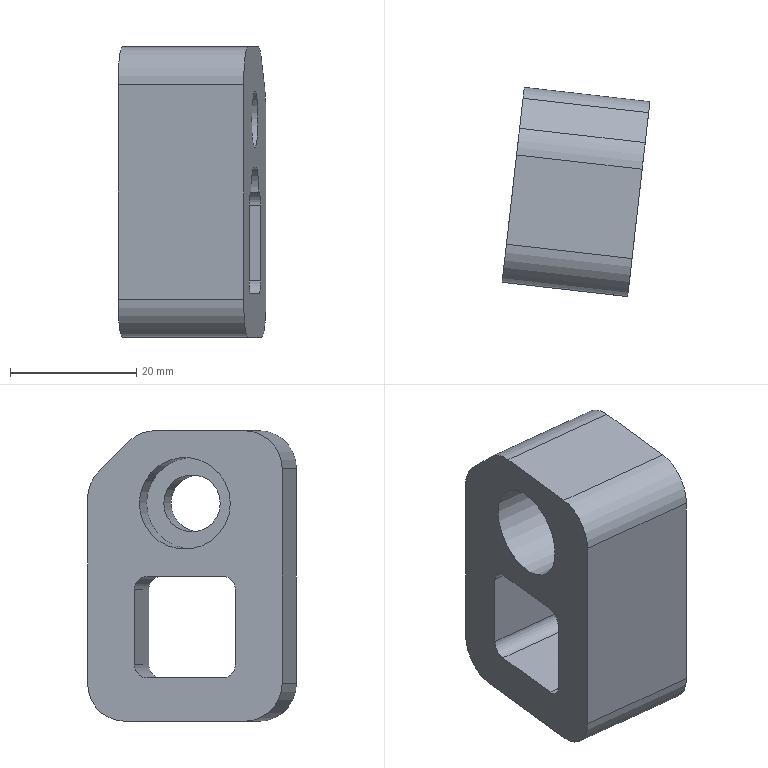Part | NX | features XQ 2 | 1 solid | 30 faces | box 23.381 x 33.065 x 46 mm | volume 19644 mm3 | plane 16 | cylinder 14 | commonest cylinder face diameters 12 x5 4.08 x4 8 x2 4 x1 9 x1 14.5 x1
STEP:
#1=CARTESIAN_POINT('',(3226.,-348.866,-101.287));
#2=VERTEX_POINT('',#1);
#3=CARTESIAN_POINT('',(3223.85,-367.744,-101.287));
#4=VERTEX_POINT('',#3);
#5=CARTESIAN_POINT('',(3230.269,-311.398,-101.287));
#6=DIRECTION('',(-0.1132,-0.9936,0.));
#7=VECTOR('',#6,1000.);
#8=LINE('',#5,#7);
#9=EDGE_CURVE('',#2,#4,#8,.T.);
#10=ORIENTED_EDGE('',*,*,#9,.T.);
#11=CARTESIAN_POINT('',(3223.17,-373.705,-95.287));
#12=VERTEX_POINT('',#11);
#13=CARTESIAN_POINT('',(3223.85,-367.744,-95.287));
#14=DIRECTION('',(-0.9936,0.1132,0.));
#15=DIRECTION('',(0.,0.,-1.));
#16=AXIS2_PLACEMENT_3D('',#13,#14,#15);
#17=CIRCLE('',#16,6.);
#18=EDGE_CURVE('',#4,#12,#17,.T.);
#19=ORIENTED_EDGE('',*,*,#18,.T.);
#20=CARTESIAN_POINT('',(3223.17,-373.705,-61.287));
#21=VERTEX_POINT('',#20);
#22=CARTESIAN_POINT('',(3223.17,-373.705,-144.775));
#23=DIRECTION('',(0.,0.,1.));
#24=VECTOR('',#23,1000.);
#25=LINE('',#22,#24);
#26=EDGE_CURVE('',#12,#21,#25,.T.);
#27=ORIENTED_EDGE('',*,*,#26,.T.);
#28=CARTESIAN_POINT('',(3223.85,-367.744,-55.287));
#29=VERTEX_POINT('',#28);
#30=CARTESIAN_POINT('',(3223.85,-367.744,-61.287));
#31=DIRECTION('',(-0.9936,0.1132,0.));
#32=DIRECTION('',(0.,0.,-1.));
#33=AXIS2_PLACEMENT_3D('',#30,#31,#32);
#34=CIRCLE('',#33,6.);
#35=EDGE_CURVE('',#21,#29,#34,.T.);
#36=ORIENTED_EDGE('',*,*,#35,.T.);
#37=CARTESIAN_POINT('',(3225.46,-353.614,-55.287));
#38=VERTEX_POINT('',#37);
#39=CARTESIAN_POINT('',(3230.269,-311.398,-55.287));
#40=DIRECTION('',(0.1132,0.9936,0.));
#41=VECTOR('',#40,1000.);
#42=LINE('',#39,#41);
#43=EDGE_CURVE('',#29,#38,#42,.T.);
#44=ORIENTED_EDGE('',*,*,#43,.T.);
#45=CARTESIAN_POINT('',(3225.94,-349.398,-57.044));
#46=VERTEX_POINT('',#45);
#47=CARTESIAN_POINT('',(3225.46,-353.614,-61.287));
#48=DIRECTION('',(-0.9936,0.1132,0.));
#49=DIRECTION('',(0.,0.,-1.));
#50=AXIS2_PLACEMENT_3D('',#47,#48,#49);
#51=CIRCLE('',#50,6.);
#52=EDGE_CURVE('',#38,#46,#51,.T.);
#53=ORIENTED_EDGE('',*,*,#52,.T.);
#54=CARTESIAN_POINT('',(3226.481,-344.651,-61.823));
#55=VERTEX_POINT('',#54);
#56=CARTESIAN_POINT('',(3233.07,-286.815,-120.033));
#57=DIRECTION('',(0.08005,0.7026,-0.7071));
#58=VECTOR('',#57,1000.);
#59=LINE('',#56,#58);
#60=EDGE_CURVE('',#46,#55,#59,.T.);
#61=ORIENTED_EDGE('',*,*,#60,.T.);
#62=CARTESIAN_POINT('',(3226.68,-342.905,-66.065));
#63=VERTEX_POINT('',#62);
#64=CARTESIAN_POINT('',(3226.,-348.866,-66.065));
#65=DIRECTION('',(-0.9936,0.1132,0.));
#66=DIRECTION('',(0.,0.,-1.));
#67=AXIS2_PLACEMENT_3D('',#64,#65,#66);
#68=CIRCLE('',#67,6.);
#69=EDGE_CURVE('',#55,#63,#68,.T.);
#70=ORIENTED_EDGE('',*,*,#69,.T.);
#71=CARTESIAN_POINT('',(3226.68,-342.905,-95.287));
#72=VERTEX_POINT('',#71);
#73=CARTESIAN_POINT('',(3226.68,-342.905,-144.775));
#74=DIRECTION('',(0.,0.,-1.));
#75=VECTOR('',#74,1000.);
#76=LINE('',#73,#75);
#77=EDGE_CURVE('',#63,#72,#76,.T.);
#78=ORIENTED_EDGE('',*,*,#77,.T.);
#79=CARTESIAN_POINT('',(3226.,-348.866,-95.287));
#80=DIRECTION('',(-0.9936,0.1132,0.));
#81=DIRECTION('',(0.,0.,-1.));
#82=AXIS2_PLACEMENT_3D('',#79,#80,#81);
#83=CIRCLE('',#82,6.);
#84=EDGE_CURVE('',#72,#2,#83,.T.);
#85=ORIENTED_EDGE('',*,*,#84,.T.);
#86=EDGE_LOOP('',(#10,#19,#27,#36,#44,#53,#61,#70,#78,#85));
#87=FACE_BOUND('',#86,.T.);
#88=CARTESIAN_POINT('',(3225.746,-351.102,-66.787));
#89=VERTEX_POINT('',#88);
#90=CARTESIAN_POINT('',(3224.925,-358.305,-66.787));
#91=DIRECTION('',(0.9936,-0.1132,0.));
#92=DIRECTION('',(0.1132,0.9936,0.));
#93=AXIS2_PLACEMENT_3D('',#90,#91,#92);
#94=CIRCLE('',#93,7.25);
#95=EDGE_CURVE('',#89,#89,#94,.T.);
#96=ORIENTED_EDGE('',*,*,#95,.T.);
#97=EDGE_LOOP('',(#96));
#98=FACE_BOUND('',#97,.T.);
#99=CARTESIAN_POINT('',(3225.604,-352.344,-78.322));
#100=VERTEX_POINT('',#99);
#101=CARTESIAN_POINT('',(3225.835,-350.317,-80.362));
#102=VERTEX_POINT('',#101);
#103=CARTESIAN_POINT('',(3225.604,-352.344,-80.362));
#104=DIRECTION('',(-0.9936,0.1132,0.));
#105=DIRECTION('',(0.,0.,-1.));
#106=AXIS2_PLACEMENT_3D('',#103,#104,#105);
#107=CIRCLE('',#106,2.04);
#108=EDGE_CURVE('',#100,#102,#107,.T.);
#109=ORIENTED_EDGE('',*,*,#108,.F.);
#110=CARTESIAN_POINT('',(3224.246,-364.266,-78.322));
#111=VERTEX_POINT('',#110);
#112=CARTESIAN_POINT('',(3230.269,-311.398,-78.322));
#113=DIRECTION('',(-0.1132,-0.9936,0.));
#114=VECTOR('',#113,1000.);
#115=LINE('',#112,#114);
#116=EDGE_CURVE('',#100,#111,#115,.T.);
#117=ORIENTED_EDGE('',*,*,#116,.T.);
#118=CARTESIAN_POINT('',(3224.015,-366.293,-80.362));
#119=VERTEX_POINT('',#118);
#120=CARTESIAN_POINT('',(3224.246,-364.266,-80.362));
#121=DIRECTION('',(-0.9936,0.1132,0.));
#122=DIRECTION('',(0.,0.,-1.));
#123=AXIS2_PLACEMENT_3D('',#120,#121,#122);
#124=CIRCLE('',#123,2.04);
#125=EDGE_CURVE('',#119,#111,#124,.T.);
#126=ORIENTED_EDGE('',*,*,#125,.F.);
#127=CARTESIAN_POINT('',(3224.015,-366.293,-92.362));
#128=VERTEX_POINT('',#127);
#129=CARTESIAN_POINT('',(3224.015,-366.293,-144.775));
#130=DIRECTION('',(0.,0.000000001,-1.));
#131=VECTOR('',#130,1000.);
#132=LINE('',#129,#131);
#133=EDGE_CURVE('',#119,#128,#132,.T.);
#134=ORIENTED_EDGE('',*,*,#133,.T.);
#135=CARTESIAN_POINT('',(3224.246,-364.266,-94.402));
#136=VERTEX_POINT('',#135);
#137=CARTESIAN_POINT('',(3224.246,-364.266,-92.362));
#138=DIRECTION('',(-0.9936,0.1132,0.));
#139=DIRECTION('',(0.,0.,-1.));
#140=AXIS2_PLACEMENT_3D('',#137,#138,#139);
#141=CIRCLE('',#140,2.04);
#142=EDGE_CURVE('',#136,#128,#141,.T.);
#143=ORIENTED_EDGE('',*,*,#142,.F.);
#144=CARTESIAN_POINT('',(3225.604,-352.344,-94.402));
#145=VERTEX_POINT('',#144);
#146=CARTESIAN_POINT('',(3230.269,-311.398,-94.402));
#147=DIRECTION('',(0.1132,0.9936,0.000000001));
#148=VECTOR('',#147,1000.);
#149=LINE('',#146,#148);
#150=EDGE_CURVE('',#136,#145,#149,.T.);
#151=ORIENTED_EDGE('',*,*,#150,.T.);
#152=CARTESIAN_POINT('',(3225.835,-350.317,-92.362));
#153=VERTEX_POINT('',#152);
#154=CARTESIAN_POINT('',(3225.604,-352.344,-92.362));
#155=DIRECTION('',(-0.9936,0.1132,0.));
#156=DIRECTION('',(0.,0.,-1.));
#157=AXIS2_PLACEMENT_3D('',#154,#155,#156);
#158=CIRCLE('',#157,2.04);
#159=EDGE_CURVE('',#153,#145,#158,.T.);
#160=ORIENTED_EDGE('',*,*,#159,.F.);
#161=CARTESIAN_POINT('',(3225.835,-350.317,-144.775));
#162=DIRECTION('',(0.,-0.000000001,1.));
#163=VECTOR('',#162,1000.);
#164=LINE('',#161,#163);
#165=EDGE_CURVE('',#153,#102,#164,.T.);
#166=ORIENTED_EDGE('',*,*,#165,.T.);
#167=EDGE_LOOP('',(#109,#117,#126,#134,#143,#151,#160,#166));
#168=FACE_BOUND('',#167,.T.);
#169=CARTESIAN_POINT('',(3230.269,-311.398,-144.775));
#170=DIRECTION('',(-0.9936,0.1132,0.));
#171=DIRECTION('',(-0.1132,-0.9936,0.));
#172=AXIS2_PLACEMENT_3D('',#169,#170,#171);
#173=PLANE('',#172);
#174=ADVANCED_FACE('',(#87,#98,#168),#173,.T.);
#175=CARTESIAN_POINT('',(3236.678,-361.154,-74.287));
#176=VERTEX_POINT('',#175);
#177=CARTESIAN_POINT('',(3236.225,-365.128,-78.322));
#178=VERTEX_POINT('',#177);
#179=CARTESIAN_POINT('',(3236.678,-361.154,-78.287));
#180=DIRECTION('',(0.9936,-0.1132,0.));
#181=DIRECTION('',(0.,0.,1.));
#182=AXIS2_PLACEMENT_3D('',#179,#180,#181);
#183=CIRCLE('',#182,4.);
#184=EDGE_CURVE('',#176,#178,#183,.T.);
#185=ORIENTED_EDGE('',*,*,#184,.T.);
#186=CARTESIAN_POINT('',(3236.452,-363.141,-78.322));
#187=VERTEX_POINT('',#186);
#188=CARTESIAN_POINT('',(3228.296,-434.719,-78.322));
#189=DIRECTION('',(0.1132,0.9936,0.));
#190=VECTOR('',#189,1000.);
#191=LINE('',#188,#190);
#192=EDGE_CURVE('',#178,#187,#191,.T.);
#193=ORIENTED_EDGE('',*,*,#192,.T.);
#194=CARTESIAN_POINT('',(3236.452,-363.141,-76.322));
#195=VERTEX_POINT('',#194);
#196=CARTESIAN_POINT('',(3236.452,-363.141,-68.563));
#197=DIRECTION('',(0.,0.,-1.));
#198=VECTOR('',#197,1000.);
#199=LINE('',#196,#198);
#200=EDGE_CURVE('',#195,#187,#199,.T.);
#201=ORIENTED_EDGE('',*,*,#200,.F.);
#202=CARTESIAN_POINT('',(3237.244,-356.186,-76.322));
#203=VERTEX_POINT('',#202);
#204=CARTESIAN_POINT('',(3237.471,-354.199,-76.322));
#205=DIRECTION('',(0.1132,0.9936,0.));
#206=VECTOR('',#205,1000.);
#207=LINE('',#204,#206);
#208=EDGE_CURVE('',#195,#203,#207,.T.);
#209=ORIENTED_EDGE('',*,*,#208,.T.);
#210=CARTESIAN_POINT('',(3237.244,-356.186,-78.322));
#211=VERTEX_POINT('',#210);
#212=CARTESIAN_POINT('',(3237.244,-356.186,-68.563));
#213=DIRECTION('',(0.,0.,-1.));
#214=VECTOR('',#213,1000.);
#215=LINE('',#212,#214);
#216=EDGE_CURVE('',#203,#211,#215,.T.);
#217=ORIENTED_EDGE('',*,*,#216,.T.);
#218=CARTESIAN_POINT('',(3237.47,-354.199,-78.322));
#219=VERTEX_POINT('',#218);
#220=CARTESIAN_POINT('',(3228.296,-434.719,-78.322));
#221=DIRECTION('',(0.1132,0.9936,0.));
#222=VECTOR('',#221,1000.);
#223=LINE('',#220,#222);
#224=EDGE_CURVE('',#211,#219,#223,.T.);
#225=ORIENTED_EDGE('',*,*,#224,.T.);
#226=CARTESIAN_POINT('',(3237.018,-358.173,-74.287));
#227=VERTEX_POINT('',#226);
#228=CARTESIAN_POINT('',(3237.018,-358.173,-78.287));
#229=DIRECTION('',(0.9936,-0.1132,0.));
#230=DIRECTION('',(0.,0.,1.));
#231=AXIS2_PLACEMENT_3D('',#228,#229,#230);
#232=CIRCLE('',#231,4.);
#233=EDGE_CURVE('',#219,#227,#232,.T.);
#234=ORIENTED_EDGE('',*,*,#233,.T.);
#235=CARTESIAN_POINT('',(3237.471,-354.199,-74.287));
#236=DIRECTION('',(-0.1132,-0.9936,0.));
#237=VECTOR('',#236,1000.);
#238=LINE('',#235,#237);
#239=EDGE_CURVE('',#227,#176,#238,.T.);
#240=ORIENTED_EDGE('',*,*,#239,.T.);
#241=EDGE_LOOP('',(#185,#193,#201,#209,#217,#225,#234,#240));
#242=FACE_BOUND('',#241,.T.);
#243=CARTESIAN_POINT('',(3228.296,-434.719,-68.563));
#244=DIRECTION('',(0.9936,-0.1132,0.));
#245=DIRECTION('',(0.1132,0.9936,0.));
#246=AXIS2_PLACEMENT_3D('',#243,#244,#245);
#247=PLANE('',#246);
#248=ADVANCED_FACE('',(#242),#247,.T.);
#249=CARTESIAN_POINT('',(3244.174,-366.034,-78.322));
#250=VERTEX_POINT('',#249);
#251=CARTESIAN_POINT('',(3283.917,-370.562,-78.322));
#252=DIRECTION('',(0.9936,-0.1132,0.));
#253=VECTOR('',#252,1000.);
#254=LINE('',#251,#253);
#255=EDGE_CURVE('',#178,#250,#254,.T.);
#256=ORIENTED_EDGE('',*,*,#255,.F.);
#257=ORIENTED_EDGE('',*,*,#184,.F.);
#258=CARTESIAN_POINT('',(3244.627,-362.059,-74.287));
#259=VERTEX_POINT('',#258);
#260=CARTESIAN_POINT('',(3284.37,-366.588,-74.287));
#261=DIRECTION('',(-0.9936,0.1132,0.));
#262=VECTOR('',#261,1000.);
#263=LINE('',#260,#262);
#264=EDGE_CURVE('',#259,#176,#263,.T.);
#265=ORIENTED_EDGE('',*,*,#264,.F.);
#266=CARTESIAN_POINT('',(3244.627,-362.059,-78.287));
#267=DIRECTION('',(-0.9936,0.1132,0.));
#268=DIRECTION('',(0.,0.,1.));
#269=AXIS2_PLACEMENT_3D('',#266,#267,#268);
#270=CIRCLE('',#269,4.);
#271=EDGE_CURVE('',#250,#259,#270,.T.);
#272=ORIENTED_EDGE('',*,*,#271,.F.);
#273=EDGE_LOOP('',(#256,#257,#265,#272));
#274=FACE_BOUND('',#273,.T.);
#275=CARTESIAN_POINT('',(3284.37,-366.588,-78.287));
#276=DIRECTION('',(0.9936,-0.1132,0.));
#277=DIRECTION('',(0.,0.,1.));
#278=AXIS2_PLACEMENT_3D('',#275,#276,#277);
#279=CYLINDRICAL_SURFACE('',#278,4.);
#280=ADVANCED_FACE('',(#274),#279,.F.);
#281=CARTESIAN_POINT('',(3245.419,-355.105,-78.322));
#282=VERTEX_POINT('',#281);
#283=CARTESIAN_POINT('',(3285.162,-359.633,-78.322));
#284=DIRECTION('',(-0.9936,0.1132,0.));
#285=VECTOR('',#284,1000.);
#286=LINE('',#283,#285);
#287=EDGE_CURVE('',#282,#219,#286,.T.);
#288=ORIENTED_EDGE('',*,*,#287,.F.);
#289=CARTESIAN_POINT('',(3244.966,-359.079,-74.287));
#290=VERTEX_POINT('',#289);
#291=CARTESIAN_POINT('',(3244.966,-359.079,-78.287));
#292=DIRECTION('',(-0.9936,0.1132,0.));
#293=DIRECTION('',(0.,0.,1.));
#294=AXIS2_PLACEMENT_3D('',#291,#292,#293);
#295=CIRCLE('',#294,4.);
#296=EDGE_CURVE('',#290,#282,#295,.T.);
#297=ORIENTED_EDGE('',*,*,#296,.F.);
#298=CARTESIAN_POINT('',(3284.709,-363.607,-74.287));
#299=DIRECTION('',(0.9936,-0.1132,0.));
#300=VECTOR('',#299,1000.);
#301=LINE('',#298,#300);
#302=EDGE_CURVE('',#227,#290,#301,.T.);
#303=ORIENTED_EDGE('',*,*,#302,.F.);
#304=ORIENTED_EDGE('',*,*,#233,.F.);
#305=EDGE_LOOP('',(#288,#297,#303,#304));
#306=FACE_BOUND('',#305,.T.);
#307=CARTESIAN_POINT('',(3284.709,-363.607,-78.287));
#308=DIRECTION('',(-0.9936,0.1132,0.));
#309=DIRECTION('',(0.,0.,-1.));
#310=AXIS2_PLACEMENT_3D('',#307,#308,#309);
#311=CYLINDRICAL_SURFACE('',#310,4.);
#312=ADVANCED_FACE('',(#306),#311,.F.);
#313=CARTESIAN_POINT('',(3245.476,-354.608,-78.322));
#314=VERTEX_POINT('',#313);
#315=CARTESIAN_POINT('',(3245.419,-355.104,-78.322));
#316=DIRECTION('',(-0.1132,-0.9936,0.));
#317=VECTOR('',#316,1000.);
#318=LINE('',#315,#317);
#319=EDGE_CURVE('',#314,#282,#318,.T.);
#320=ORIENTED_EDGE('',*,*,#319,.F.);
#321=CARTESIAN_POINT('',(3245.707,-352.581,-80.362));
#322=VERTEX_POINT('',#321);
#323=CARTESIAN_POINT('',(3245.476,-354.608,-80.362));
#324=DIRECTION('',(-0.9936,0.1132,0.));
#325=DIRECTION('',(0.,0.,1.));
#326=AXIS2_PLACEMENT_3D('',#323,#324,#325);
#327=CIRCLE('',#326,2.04);
#328=EDGE_CURVE('',#314,#322,#327,.T.);
#329=ORIENTED_EDGE('',*,*,#328,.T.);
#330=CARTESIAN_POINT('',(3245.707,-352.581,-92.362));
#331=VERTEX_POINT('',#330);
#332=CARTESIAN_POINT('',(3245.707,-352.581,-92.362));
#333=DIRECTION('',(0.,-0.000000001,1.));
#334=VECTOR('',#333,1000.);
#335=LINE('',#332,#334);
#336=EDGE_CURVE('',#331,#322,#335,.T.);
#337=ORIENTED_EDGE('',*,*,#336,.F.);
#338=CARTESIAN_POINT('',(3245.476,-354.608,-94.402));
#339=VERTEX_POINT('',#338);
#340=CARTESIAN_POINT('',(3245.476,-354.608,-92.362));
#341=DIRECTION('',(-0.9936,0.1132,0.));
#342=DIRECTION('',(0.,0.,1.));
#343=AXIS2_PLACEMENT_3D('',#340,#341,#342);
#344=CIRCLE('',#343,2.04);
#345=EDGE_CURVE('',#331,#339,#344,.T.);
#346=ORIENTED_EDGE('',*,*,#345,.T.);
#347=CARTESIAN_POINT('',(3244.117,-366.531,-94.402));
#348=VERTEX_POINT('',#347);
#349=CARTESIAN_POINT('',(3244.117,-366.531,-94.402));
#350=DIRECTION('',(0.1132,0.9936,0.000000001));
#351=VECTOR('',#350,1000.);
#352=LINE('',#349,#351);
#353=EDGE_CURVE('',#348,#339,#352,.T.);
#354=ORIENTED_EDGE('',*,*,#353,.F.);
#355=CARTESIAN_POINT('',(3243.886,-368.557,-92.362));
#356=VERTEX_POINT('',#355);
#357=CARTESIAN_POINT('',(3244.117,-366.531,-92.362));
#358=DIRECTION('',(-0.9936,0.1132,0.));
#359=DIRECTION('',(0.,0.,1.));
#360=AXIS2_PLACEMENT_3D('',#357,#358,#359);
#361=CIRCLE('',#360,2.04);
#362=EDGE_CURVE('',#348,#356,#361,.T.);
#363=ORIENTED_EDGE('',*,*,#362,.T.);
#364=CARTESIAN_POINT('',(3243.886,-368.557,-80.362));
#365=VERTEX_POINT('',#364);
#366=CARTESIAN_POINT('',(3243.886,-368.557,-80.362));
#367=DIRECTION('',(0.,0.000000001,-1.));
#368=VECTOR('',#367,1000.);
#369=LINE('',#366,#368);
#370=EDGE_CURVE('',#365,#356,#369,.T.);
#371=ORIENTED_EDGE('',*,*,#370,.F.);
#372=CARTESIAN_POINT('',(3244.117,-366.531,-78.322));
#373=VERTEX_POINT('',#372);
#374=CARTESIAN_POINT('',(3244.117,-366.531,-80.362));
#375=DIRECTION('',(-0.9936,0.1132,0.));
#376=DIRECTION('',(0.,0.,1.));
#377=AXIS2_PLACEMENT_3D('',#374,#375,#376);
#378=CIRCLE('',#377,2.04);
#379=EDGE_CURVE('',#365,#373,#378,.T.);
#380=ORIENTED_EDGE('',*,*,#379,.T.);
#381=CARTESIAN_POINT('',(3245.419,-355.104,-78.322));
#382=DIRECTION('',(-0.1132,-0.9936,0.));
#383=VECTOR('',#382,1000.);
#384=LINE('',#381,#383);
#385=EDGE_CURVE('',#250,#373,#384,.T.);
#386=ORIENTED_EDGE('',*,*,#385,.F.);
#387=ORIENTED_EDGE('',*,*,#271,.T.);
#388=CARTESIAN_POINT('',(3245.419,-355.104,-74.287));
#389=DIRECTION('',(-0.1132,-0.9936,0.));
#390=VECTOR('',#389,1000.);
#391=LINE('',#388,#390);
#392=EDGE_CURVE('',#290,#259,#391,.T.);
#393=ORIENTED_EDGE('',*,*,#392,.F.);
#394=ORIENTED_EDGE('',*,*,#296,.T.);
#395=EDGE_LOOP('',(#320,#329,#337,#346,#354,#363,#371,#380,#386,#387,#393,#394));
#396=FACE_BOUND('',#395,.T.);
#397=CARTESIAN_POINT('',(3243.042,-375.969,-61.287));
#398=VERTEX_POINT('',#397);
#399=CARTESIAN_POINT('',(3243.042,-375.969,-95.287));
#400=VERTEX_POINT('',#399);
#401=CARTESIAN_POINT('',(3243.042,-375.969,-68.563));
#402=DIRECTION('',(0.,0.,-1.));
#403=VECTOR('',#402,1000.);
#404=LINE('',#401,#403);
#405=EDGE_CURVE('',#398,#400,#404,.T.);
#406=ORIENTED_EDGE('',*,*,#405,.T.);
#407=CARTESIAN_POINT('',(3243.721,-370.008,-101.287));
#408=VERTEX_POINT('',#407);
#409=CARTESIAN_POINT('',(3243.721,-370.008,-95.287));
#410=DIRECTION('',(0.9936,-0.1132,0.));
#411=DIRECTION('',(0.,0.,1.));
#412=AXIS2_PLACEMENT_3D('',#409,#410,#411);
#413=CIRCLE('',#412,6.);
#414=EDGE_CURVE('',#400,#408,#413,.T.);
#415=ORIENTED_EDGE('',*,*,#414,.T.);
#416=CARTESIAN_POINT('',(3245.872,-351.13,-101.287));
#417=VERTEX_POINT('',#416);
#418=CARTESIAN_POINT('',(3236.245,-435.624,-101.287));
#419=DIRECTION('',(0.1132,0.9936,0.));
#420=VECTOR('',#419,1000.);
#421=LINE('',#418,#420);
#422=EDGE_CURVE('',#408,#417,#421,.T.);
#423=ORIENTED_EDGE('',*,*,#422,.T.);
#424=CARTESIAN_POINT('',(3246.551,-345.169,-95.287));
#425=VERTEX_POINT('',#424);
#426=CARTESIAN_POINT('',(3245.872,-351.13,-95.287));
#427=DIRECTION('',(0.9936,-0.1132,0.));
#428=DIRECTION('',(0.,0.,1.));
#429=AXIS2_PLACEMENT_3D('',#426,#427,#428);
#430=CIRCLE('',#429,6.);
#431=EDGE_CURVE('',#417,#425,#430,.T.);
#432=ORIENTED_EDGE('',*,*,#431,.T.);
#433=CARTESIAN_POINT('',(3246.551,-345.169,-66.065));
#434=VERTEX_POINT('',#433);
#435=CARTESIAN_POINT('',(3246.551,-345.169,-68.563));
#436=DIRECTION('',(0.,0.,1.));
#437=VECTOR('',#436,1000.);
#438=LINE('',#435,#437);
#439=EDGE_CURVE('',#425,#434,#438,.T.);
#440=ORIENTED_EDGE('',*,*,#439,.T.);
#441=CARTESIAN_POINT('',(3246.352,-346.915,-61.823));
#442=VERTEX_POINT('',#441);
#443=CARTESIAN_POINT('',(3245.872,-351.13,-66.065));
#444=DIRECTION('',(0.9936,-0.1132,0.));
#445=DIRECTION('',(0.,0.,1.));
#446=AXIS2_PLACEMENT_3D('',#443,#444,#445);
#447=CIRCLE('',#446,6.);
#448=EDGE_CURVE('',#434,#442,#447,.T.);
#449=ORIENTED_EDGE('',*,*,#448,.T.);
#450=CARTESIAN_POINT('',(3245.811,-351.662,-57.044));
#451=VERTEX_POINT('',#450);
#452=CARTESIAN_POINT('',(3241.68,-387.921,-20.551));
#453=DIRECTION('',(-0.08005,-0.7026,0.7071));
#454=VECTOR('',#453,1000.);
#455=LINE('',#452,#454);
#456=EDGE_CURVE('',#442,#451,#455,.T.);
#457=ORIENTED_EDGE('',*,*,#456,.T.);
#458=CARTESIAN_POINT('',(3245.331,-355.878,-55.287));
#459=VERTEX_POINT('',#458);
#460=CARTESIAN_POINT('',(3245.331,-355.878,-61.287));
#461=DIRECTION('',(0.9936,-0.1132,0.));
#462=DIRECTION('',(0.,0.,1.));
#463=AXIS2_PLACEMENT_3D('',#460,#461,#462);
#464=CIRCLE('',#463,6.);
#465=EDGE_CURVE('',#451,#459,#464,.T.);
#466=ORIENTED_EDGE('',*,*,#465,.T.);
#467=CARTESIAN_POINT('',(3243.721,-370.008,-55.287));
#468=VERTEX_POINT('',#467);
#469=CARTESIAN_POINT('',(3236.245,-435.624,-55.287));
#470=DIRECTION('',(-0.1132,-0.9936,0.));
#471=VECTOR('',#470,1000.);
#472=LINE('',#469,#471);
#473=EDGE_CURVE('',#459,#468,#472,.T.);
#474=ORIENTED_EDGE('',*,*,#473,.T.);
#475=CARTESIAN_POINT('',(3243.721,-370.008,-61.287));
#476=DIRECTION('',(0.9936,-0.1132,0.));
#477=DIRECTION('',(0.,0.,1.));
#478=AXIS2_PLACEMENT_3D('',#475,#476,#477);
#479=CIRCLE('',#478,6.);
#480=EDGE_CURVE('',#468,#398,#479,.T.);
#481=ORIENTED_EDGE('',*,*,#480,.T.);
#482=EDGE_LOOP('',(#406,#415,#423,#432,#440,#449,#457,#466,#474,#481));
#483=FACE_BOUND('',#482,.T.);
#484=CARTESIAN_POINT('',(3244.287,-365.04,-66.787));
#485=VERTEX_POINT('',#484);
#486=CARTESIAN_POINT('',(3244.796,-360.569,-66.787));
#487=DIRECTION('',(0.9936,-0.1132,0.));
#488=DIRECTION('',(-0.1132,-0.9936,0.));
#489=AXIS2_PLACEMENT_3D('',#486,#487,#488);
#490=CIRCLE('',#489,4.5);
#491=EDGE_CURVE('',#485,#485,#490,.T.);
#492=ORIENTED_EDGE('',*,*,#491,.F.);
#493=EDGE_LOOP('',(#492));
#494=FACE_BOUND('',#493,.T.);
#495=CARTESIAN_POINT('',(3236.245,-435.624,-68.563));
#496=DIRECTION('',(0.9936,-0.1132,0.));
#497=DIRECTION('',(0.1132,0.9936,0.));
#498=AXIS2_PLACEMENT_3D('',#495,#496,#497);
#499=PLANE('',#498);
#500=ADVANCED_FACE('',(#396,#483,#494),#499,.T.);
#501=ORIENTED_EDGE('',*,*,#422,.F.);
#502=CARTESIAN_POINT('',(3218.882,-367.178,-101.287));
#503=DIRECTION('',(-0.9936,0.1132,0.));
#504=VECTOR('',#503,1000.);
#505=LINE('',#502,#504);
#506=EDGE_CURVE('',#408,#4,#505,.T.);
#507=ORIENTED_EDGE('',*,*,#506,.T.);
#508=ORIENTED_EDGE('',*,*,#9,.F.);
#509=CARTESIAN_POINT('',(3221.033,-348.3,-101.287));
#510=DIRECTION('',(0.9936,-0.1132,0.));
#511=VECTOR('',#510,1000.);
#512=LINE('',#509,#511);
#513=EDGE_CURVE('',#2,#417,#512,.T.);
#514=ORIENTED_EDGE('',*,*,#513,.T.);
#515=EDGE_LOOP('',(#501,#507,#508,#514));
#516=FACE_BOUND('',#515,.T.);
#517=CARTESIAN_POINT('',(3219.957,-357.739,-101.287));
#518=DIRECTION('',(0.,0.,-1.));
#519=DIRECTION('',(-0.9588,0.284,0.));
#520=AXIS2_PLACEMENT_3D('',#517,#518,#519);
#521=PLANE('',#520);
#522=ADVANCED_FACE('',(#516),#521,.T.);
#523=ORIENTED_EDGE('',*,*,#26,.F.);
#524=CARTESIAN_POINT('',(3218.203,-373.139,-95.287));
#525=DIRECTION('',(0.9936,-0.1132,0.));
#526=VECTOR('',#525,1000.);
#527=LINE('',#524,#526);
#528=EDGE_CURVE('',#12,#400,#527,.T.);
#529=ORIENTED_EDGE('',*,*,#528,.T.);
#530=ORIENTED_EDGE('',*,*,#405,.F.);
#531=CARTESIAN_POINT('',(3218.203,-373.139,-61.287));
#532=DIRECTION('',(-0.9936,0.1132,0.));
#533=VECTOR('',#532,1000.);
#534=LINE('',#531,#533);
#535=EDGE_CURVE('',#398,#21,#534,.T.);
#536=ORIENTED_EDGE('',*,*,#535,.T.);
#537=EDGE_LOOP('',(#523,#529,#530,#536));
#538=FACE_BOUND('',#537,.T.);
#539=CARTESIAN_POINT('',(3218.203,-373.139,-86.362));
#540=DIRECTION('',(-0.1132,-0.9936,0.));
#541=DIRECTION('',(0.9936,-0.1132,0.));
#542=AXIS2_PLACEMENT_3D('',#539,#540,#541);
#543=PLANE('',#542);
#544=ADVANCED_FACE('',(#538),#543,.T.);
#545=ORIENTED_EDGE('',*,*,#439,.F.);
#546=CARTESIAN_POINT('',(3221.712,-342.339,-95.287));
#547=DIRECTION('',(-0.9936,0.1132,0.));
#548=VECTOR('',#547,1000.);
#549=LINE('',#546,#548);
#550=EDGE_CURVE('',#425,#72,#549,.T.);
#551=ORIENTED_EDGE('',*,*,#550,.T.);
#552=ORIENTED_EDGE('',*,*,#77,.F.);
#553=CARTESIAN_POINT('',(3221.712,-342.339,-66.065));
#554=DIRECTION('',(0.9936,-0.1132,0.));
#555=VECTOR('',#554,1000.);
#556=LINE('',#553,#555);
#557=EDGE_CURVE('',#63,#434,#556,.T.);
#558=ORIENTED_EDGE('',*,*,#557,.T.);
#559=EDGE_LOOP('',(#545,#551,#552,#558));
#560=FACE_BOUND('',#559,.T.);
#561=CARTESIAN_POINT('',(3221.712,-342.339,-86.362));
#562=DIRECTION('',(0.1132,0.9936,0.));
#563=DIRECTION('',(-0.9936,0.1132,0.));
#564=AXIS2_PLACEMENT_3D('',#561,#562,#563);
#565=PLANE('',#564);
#566=ADVANCED_FACE('',(#560),#565,.T.);
#567=ORIENTED_EDGE('',*,*,#473,.F.);
#568=CARTESIAN_POINT('',(3220.492,-353.048,-55.287));
#569=DIRECTION('',(-0.9936,0.1132,0.));
#570=VECTOR('',#569,1000.);
#571=LINE('',#568,#570);
#572=EDGE_CURVE('',#459,#38,#571,.T.);
#573=ORIENTED_EDGE('',*,*,#572,.T.);
#574=ORIENTED_EDGE('',*,*,#43,.F.);
#575=CARTESIAN_POINT('',(3218.882,-367.178,-55.287));
#576=DIRECTION('',(0.9936,-0.1132,0.));
#577=VECTOR('',#576,1000.);
#578=LINE('',#575,#577);
#579=EDGE_CURVE('',#29,#468,#578,.T.);
#580=ORIENTED_EDGE('',*,*,#579,.T.);
#581=EDGE_LOOP('',(#567,#573,#574,#580));
#582=FACE_BOUND('',#581,.T.);
#583=CARTESIAN_POINT('',(3219.957,-357.739,-55.287));
#584=DIRECTION('',(0.,0.,1.));
#585=DIRECTION('',(0.9588,-0.284,0.));
#586=AXIS2_PLACEMENT_3D('',#583,#584,#585);
#587=PLANE('',#586);
#588=ADVANCED_FACE('',(#582),#587,.T.);
#589=ORIENTED_EDGE('',*,*,#456,.F.);
#590=CARTESIAN_POINT('',(3221.513,-344.085,-61.823));
#591=DIRECTION('',(-0.9936,0.1132,0.));
#592=VECTOR('',#591,1000.);
#593=LINE('',#590,#592);
#594=EDGE_CURVE('',#442,#55,#593,.T.);
#595=ORIENTED_EDGE('',*,*,#594,.T.);
#596=ORIENTED_EDGE('',*,*,#60,.F.);
#597=CARTESIAN_POINT('',(3220.972,-348.832,-57.044));
#598=DIRECTION('',(0.9936,-0.1132,0.));
#599=VECTOR('',#598,1000.);
#600=LINE('',#597,#599);
#601=EDGE_CURVE('',#46,#451,#600,.T.);
#602=ORIENTED_EDGE('',*,*,#601,.T.);
#603=EDGE_LOOP('',(#589,#595,#596,#602));
#604=FACE_BOUND('',#603,.T.);
#605=CARTESIAN_POINT('',(3221.469,-344.471,-61.433));
#606=DIRECTION('',(-0.08005,-0.7026,-0.7071));
#607=DIRECTION('',(0.9936,-0.1132,0.));
#608=AXIS2_PLACEMENT_3D('',#605,#606,#607);
#609=PLANE('',#608);
#610=ADVANCED_FACE('',(#604),#609,.F.);
#611=ORIENTED_EDGE('',*,*,#18,.F.);
#612=ORIENTED_EDGE('',*,*,#506,.F.);
#613=ORIENTED_EDGE('',*,*,#414,.F.);
#614=ORIENTED_EDGE('',*,*,#528,.F.);
#615=EDGE_LOOP('',(#611,#612,#613,#614));
#616=FACE_BOUND('',#615,.T.);
#617=CARTESIAN_POINT('',(3218.882,-367.178,-95.287));
#618=DIRECTION('',(-0.9936,0.1132,0.));
#619=DIRECTION('',(0.,0.,-1.));
#620=AXIS2_PLACEMENT_3D('',#617,#618,#619);
#621=CYLINDRICAL_SURFACE('',#620,6.);
#622=ADVANCED_FACE('',(#616),#621,.T.);
#623=ORIENTED_EDGE('',*,*,#431,.F.);
#624=ORIENTED_EDGE('',*,*,#513,.F.);
#625=ORIENTED_EDGE('',*,*,#84,.F.);
#626=ORIENTED_EDGE('',*,*,#550,.F.);
#627=EDGE_LOOP('',(#623,#624,#625,#626));
#628=FACE_BOUND('',#627,.T.);
#629=CARTESIAN_POINT('',(3221.033,-348.3,-95.287));
#630=DIRECTION('',(0.9936,-0.1132,0.));
#631=DIRECTION('',(0.,0.,1.));
#632=AXIS2_PLACEMENT_3D('',#629,#630,#631);
#633=CYLINDRICAL_SURFACE('',#632,6.);
#634=ADVANCED_FACE('',(#628),#633,.T.);
#635=ORIENTED_EDGE('',*,*,#69,.F.);
#636=ORIENTED_EDGE('',*,*,#594,.F.);
#637=ORIENTED_EDGE('',*,*,#448,.F.);
#638=ORIENTED_EDGE('',*,*,#557,.F.);
#639=EDGE_LOOP('',(#635,#636,#637,#638));
#640=FACE_BOUND('',#639,.T.);
#641=CARTESIAN_POINT('',(3221.033,-348.3,-66.065));
#642=DIRECTION('',(0.9936,-0.1132,0.));
#643=DIRECTION('',(0.,0.,1.));
#644=AXIS2_PLACEMENT_3D('',#641,#642,#643);
#645=CYLINDRICAL_SURFACE('',#644,6.);
#646=ADVANCED_FACE('',(#640),#645,.T.);
#647=ORIENTED_EDGE('',*,*,#465,.F.);
#648=ORIENTED_EDGE('',*,*,#601,.F.);
#649=ORIENTED_EDGE('',*,*,#52,.F.);
#650=ORIENTED_EDGE('',*,*,#572,.F.);
#651=EDGE_LOOP('',(#647,#648,#649,#650));
#652=FACE_BOUND('',#651,.T.);
#653=CARTESIAN_POINT('',(3220.492,-353.048,-61.287));
#654=DIRECTION('',(-0.9936,0.1132,0.));
#655=DIRECTION('',(0.,0.,-1.));
#656=AXIS2_PLACEMENT_3D('',#653,#654,#655);
#657=CYLINDRICAL_SURFACE('',#656,6.);
#658=ADVANCED_FACE('',(#652),#657,.T.);
#659=ORIENTED_EDGE('',*,*,#35,.F.);
#660=ORIENTED_EDGE('',*,*,#535,.F.);
#661=ORIENTED_EDGE('',*,*,#480,.F.);
#662=ORIENTED_EDGE('',*,*,#579,.F.);
#663=EDGE_LOOP('',(#659,#660,#661,#662));
#664=FACE_BOUND('',#663,.T.);
#665=CARTESIAN_POINT('',(3218.882,-367.178,-61.287));
#666=DIRECTION('',(-0.9936,0.1132,0.));
#667=DIRECTION('',(0.,0.,-1.));
#668=AXIS2_PLACEMENT_3D('',#665,#666,#667);
#669=CYLINDRICAL_SURFACE('',#668,6.);
#670=ADVANCED_FACE('',(#664),#669,.T.);
#671=ORIENTED_EDGE('',*,*,#491,.T.);
#672=EDGE_LOOP('',(#671));
#673=FACE_BOUND('',#672,.T.);
#674=CARTESIAN_POINT('',(3234.351,-363.908,-66.787));
#675=VERTEX_POINT('',#674);
#676=CARTESIAN_POINT('',(3234.861,-359.437,-66.787));
#677=DIRECTION('',(0.9936,-0.1132,0.));
#678=DIRECTION('',(-0.1132,-0.9936,0.));
#679=AXIS2_PLACEMENT_3D('',#676,#677,#678);
#680=CIRCLE('',#679,4.5);
#681=EDGE_CURVE('',#675,#675,#680,.T.);
#682=ORIENTED_EDGE('',*,*,#681,.F.);
#683=EDGE_LOOP('',(#682));
#684=FACE_BOUND('',#683,.T.);
#685=CARTESIAN_POINT('',(3219.957,-357.739,-66.787));
#686=DIRECTION('',(0.9936,-0.1132,0.));
#687=DIRECTION('',(-0.01966,-0.1725,-0.9848));
#688=AXIS2_PLACEMENT_3D('',#685,#686,#687);
#689=CYLINDRICAL_SURFACE('',#688,4.5);
#690=ADVANCED_FACE('',(#673,#684),#689,.F.);
#691=ORIENTED_EDGE('',*,*,#681,.T.);
#692=EDGE_LOOP('',(#691));
#693=FACE_BOUND('',#692,.T.);
#694=CARTESIAN_POINT('',(3234.04,-366.64,-66.787));
#695=VERTEX_POINT('',#694);
#696=CARTESIAN_POINT('',(3234.861,-359.437,-66.787));
#697=DIRECTION('',(0.9936,-0.1132,0.));
#698=DIRECTION('',(-0.1132,-0.9936,0.));
#699=AXIS2_PLACEMENT_3D('',#696,#697,#698);
#700=CIRCLE('',#699,7.25);
#701=EDGE_CURVE('',#695,#695,#700,.T.);
#702=ORIENTED_EDGE('',*,*,#701,.F.);
#703=EDGE_LOOP('',(#702));
#704=FACE_BOUND('',#703,.T.);
#705=CARTESIAN_POINT('',(3234.861,-359.437,-66.787));
#706=DIRECTION('',(0.9936,-0.1132,0.));
#707=DIRECTION('',(0.1132,0.9936,0.));
#708=AXIS2_PLACEMENT_3D('',#705,#706,#707);
#709=PLANE('',#708);
#710=ADVANCED_FACE('',(#693,#704),#709,.F.);
#711=ORIENTED_EDGE('',*,*,#701,.T.);
#712=EDGE_LOOP('',(#711));
#713=FACE_BOUND('',#712,.T.);
#714=ORIENTED_EDGE('',*,*,#95,.F.);
#715=EDGE_LOOP('',(#714));
#716=FACE_BOUND('',#715,.T.);
#717=CARTESIAN_POINT('',(3219.957,-357.739,-66.787));
#718=DIRECTION('',(0.9936,-0.1132,0.));
#719=DIRECTION('',(-0.01966,-0.1725,-0.9848));
#720=AXIS2_PLACEMENT_3D('',#717,#718,#719);
#721=CYLINDRICAL_SURFACE('',#720,7.25);
#722=ADVANCED_FACE('',(#713,#716),#721,.F.);
#723=ORIENTED_EDGE('',*,*,#392,.T.);
#724=ORIENTED_EDGE('',*,*,#264,.T.);
#725=ORIENTED_EDGE('',*,*,#239,.F.);
#726=ORIENTED_EDGE('',*,*,#302,.T.);
#727=EDGE_LOOP('',(#723,#724,#725,#726));
#728=FACE_BOUND('',#727,.T.);
#729=CARTESIAN_POINT('',(3285.162,-359.633,-74.287));
#730=DIRECTION('',(0.,0.,-1.));
#731=DIRECTION('',(-0.9936,0.1132,0.));
#732=AXIS2_PLACEMENT_3D('',#729,#730,#731);
#733=PLANE('',#732);
#734=ADVANCED_FACE('',(#728),#733,.T.);
#735=CARTESIAN_POINT('',(3285.219,-359.136,-78.322));
#736=DIRECTION('',(0.9936,-0.1132,0.));
#737=VECTOR('',#736,1000.);
#738=LINE('',#735,#737);
#739=EDGE_CURVE('',#100,#314,#738,.T.);
#740=ORIENTED_EDGE('',*,*,#739,.T.);
#741=ORIENTED_EDGE('',*,*,#319,.T.);
#742=ORIENTED_EDGE('',*,*,#287,.T.);
#743=ORIENTED_EDGE('',*,*,#224,.F.);
#744=CARTESIAN_POINT('',(3235.257,-355.96,-78.322));
#745=VERTEX_POINT('',#744);
#746=CARTESIAN_POINT('',(3284.936,-361.62,-78.322));
#747=DIRECTION('',(0.9936,-0.1132,0.));
#748=VECTOR('',#747,1000.);
#749=LINE('',#746,#748);
#750=EDGE_CURVE('',#745,#211,#749,.T.);
#751=ORIENTED_EDGE('',*,*,#750,.F.);
#752=CARTESIAN_POINT('',(3234.465,-362.915,-78.322));
#753=VERTEX_POINT('',#752);
#754=CARTESIAN_POINT('',(3235.483,-353.972,-78.322));
#755=DIRECTION('',(-0.1132,-0.9936,0.));
#756=VECTOR('',#755,1000.);
#757=LINE('',#754,#756);
#758=EDGE_CURVE('',#745,#753,#757,.T.);
#759=ORIENTED_EDGE('',*,*,#758,.T.);
#760=CARTESIAN_POINT('',(3284.143,-368.575,-78.322));
#761=DIRECTION('',(0.9936,-0.1132,0.));
#762=VECTOR('',#761,1000.);
#763=LINE('',#760,#762);
#764=EDGE_CURVE('',#753,#187,#763,.T.);
#765=ORIENTED_EDGE('',*,*,#764,.T.);
#766=ORIENTED_EDGE('',*,*,#192,.F.);
#767=ORIENTED_EDGE('',*,*,#255,.T.);
#768=ORIENTED_EDGE('',*,*,#385,.T.);
#769=CARTESIAN_POINT('',(3193.445,-360.757,-78.322));
#770=DIRECTION('',(0.9936,-0.1132,0.));
#771=VECTOR('',#770,1000.);
#772=LINE('',#769,#771);
#773=EDGE_CURVE('',#111,#373,#772,.T.);
#774=ORIENTED_EDGE('',*,*,#773,.F.);
#775=ORIENTED_EDGE('',*,*,#116,.F.);
#776=EDGE_LOOP('',(#740,#741,#742,#743,#751,#759,#765,#766,#767,#768,#774,#775));
#777=FACE_BOUND('',#776,.T.);
#778=CARTESIAN_POINT('',(3285.162,-359.633,-78.322));
#779=DIRECTION('',(0.,0.,-1.));
#780=DIRECTION('',(-0.9936,0.1132,0.));
#781=AXIS2_PLACEMENT_3D('',#778,#779,#780);
#782=PLANE('',#781);
#783=ADVANCED_FACE('',(#777),#782,.T.);
#784=ORIENTED_EDGE('',*,*,#125,.T.);
#785=ORIENTED_EDGE('',*,*,#773,.T.);
#786=ORIENTED_EDGE('',*,*,#379,.F.);
#787=CARTESIAN_POINT('',(3193.214,-362.784,-80.362));
#788=DIRECTION('',(0.9936,-0.1132,0.));
#789=VECTOR('',#788,1000.);
#790=LINE('',#787,#789);
#791=EDGE_CURVE('',#119,#365,#790,.T.);
#792=ORIENTED_EDGE('',*,*,#791,.F.);
#793=EDGE_LOOP('',(#784,#785,#786,#792));
#794=FACE_BOUND('',#793,.T.);
#795=CARTESIAN_POINT('',(3193.445,-360.757,-80.362));
#796=DIRECTION('',(-0.9936,0.1132,0.));
#797=DIRECTION('',(0.,0.,1.));
#798=AXIS2_PLACEMENT_3D('',#795,#796,#797);
#799=CYLINDRICAL_SURFACE('',#798,2.04);
#800=ADVANCED_FACE('',(#794),#799,.F.);
#801=ORIENTED_EDGE('',*,*,#791,.T.);
#802=ORIENTED_EDGE('',*,*,#370,.T.);
#803=CARTESIAN_POINT('',(3193.214,-362.784,-92.362));
#804=DIRECTION('',(0.9936,-0.1132,0.));
#805=VECTOR('',#804,1000.);
#806=LINE('',#803,#805);
#807=EDGE_CURVE('',#128,#356,#806,.T.);
#808=ORIENTED_EDGE('',*,*,#807,.F.);
#809=ORIENTED_EDGE('',*,*,#133,.F.);
#810=EDGE_LOOP('',(#801,#802,#808,#809));
#811=FACE_BOUND('',#810,.T.);
#812=CARTESIAN_POINT('',(3193.214,-362.784,-80.362));
#813=DIRECTION('',(0.1132,0.9936,0.000000001));
#814=DIRECTION('',(0.1125,-0.01281,-0.9936));
#815=AXIS2_PLACEMENT_3D('',#812,#813,#814);
#816=PLANE('',#815);
#817=ADVANCED_FACE('',(#811),#816,.T.);
#818=ORIENTED_EDGE('',*,*,#142,.T.);
#819=ORIENTED_EDGE('',*,*,#807,.T.);
#820=ORIENTED_EDGE('',*,*,#362,.F.);
#821=CARTESIAN_POINT('',(3193.445,-360.757,-94.402));
#822=DIRECTION('',(0.9936,-0.1132,0.));
#823=VECTOR('',#822,1000.);
#824=LINE('',#821,#823);
#825=EDGE_CURVE('',#136,#348,#824,.T.);
#826=ORIENTED_EDGE('',*,*,#825,.F.);
#827=EDGE_LOOP('',(#818,#819,#820,#826));
#828=FACE_BOUND('',#827,.T.);
#829=CARTESIAN_POINT('',(3193.445,-360.757,-92.362));
#830=DIRECTION('',(-0.9936,0.1132,0.));
#831=DIRECTION('',(0.,0.,1.));
#832=AXIS2_PLACEMENT_3D('',#829,#830,#831);
#833=CYLINDRICAL_SURFACE('',#832,2.04);
#834=ADVANCED_FACE('',(#828),#833,.F.);
#835=ORIENTED_EDGE('',*,*,#825,.T.);
#836=ORIENTED_EDGE('',*,*,#353,.T.);
#837=CARTESIAN_POINT('',(3194.804,-348.834,-94.402));
#838=DIRECTION('',(0.9936,-0.1132,0.));
#839=VECTOR('',#838,1000.);
#840=LINE('',#837,#839);
#841=EDGE_CURVE('',#145,#339,#840,.T.);
#842=ORIENTED_EDGE('',*,*,#841,.F.);
#843=ORIENTED_EDGE('',*,*,#150,.F.);
#844=EDGE_LOOP('',(#835,#836,#842,#843));
#845=FACE_BOUND('',#844,.T.);
#846=CARTESIAN_POINT('',(3193.445,-360.757,-94.402));
#847=DIRECTION('',(0.,-0.000000002,1.));
#848=DIRECTION('',(0.9936,-0.1132,0.));
#849=AXIS2_PLACEMENT_3D('',#846,#847,#848);
#850=PLANE('',#849);
#851=ADVANCED_FACE('',(#845),#850,.T.);
#852=ORIENTED_EDGE('',*,*,#159,.T.);
#853=ORIENTED_EDGE('',*,*,#841,.T.);
#854=ORIENTED_EDGE('',*,*,#345,.F.);
#855=CARTESIAN_POINT('',(3195.034,-346.807,-92.362));
#856=DIRECTION('',(0.9936,-0.1132,0.));
#857=VECTOR('',#856,1000.);
#858=LINE('',#855,#857);
#859=EDGE_CURVE('',#153,#331,#858,.T.);
#860=ORIENTED_EDGE('',*,*,#859,.F.);
#861=EDGE_LOOP('',(#852,#853,#854,#860));
#862=FACE_BOUND('',#861,.T.);
#863=CARTESIAN_POINT('',(3194.804,-348.834,-92.362));
#864=DIRECTION('',(-0.9936,0.1132,0.));
#865=DIRECTION('',(0.,0.,1.));
#866=AXIS2_PLACEMENT_3D('',#863,#864,#865);
#867=CYLINDRICAL_SURFACE('',#866,2.04);
#868=ADVANCED_FACE('',(#862),#867,.F.);
#869=ORIENTED_EDGE('',*,*,#859,.T.);
#870=ORIENTED_EDGE('',*,*,#336,.T.);
#871=CARTESIAN_POINT('',(3285.449,-357.109,-80.362));
#872=DIRECTION('',(0.9936,-0.1132,0.));
#873=VECTOR('',#872,1000.);
#874=LINE('',#871,#873);
#875=EDGE_CURVE('',#102,#322,#874,.T.);
#876=ORIENTED_EDGE('',*,*,#875,.F.);
#877=ORIENTED_EDGE('',*,*,#165,.F.);
#878=EDGE_LOOP('',(#869,#870,#876,#877));
#879=FACE_BOUND('',#878,.T.);
#880=CARTESIAN_POINT('',(3195.034,-346.807,-92.362));
#881=DIRECTION('',(-0.1132,-0.9936,-0.000000001));
#882=DIRECTION('',(-0.1125,0.01281,0.9936));
#883=AXIS2_PLACEMENT_3D('',#880,#881,#882);
#884=PLANE('',#883);
#885=ADVANCED_FACE('',(#879),#884,.T.);
#886=ORIENTED_EDGE('',*,*,#108,.T.);
#887=ORIENTED_EDGE('',*,*,#875,.T.);
#888=ORIENTED_EDGE('',*,*,#328,.F.);
#889=ORIENTED_EDGE('',*,*,#739,.F.);
#890=EDGE_LOOP('',(#886,#887,#888,#889));
#891=FACE_BOUND('',#890,.T.);
#892=CARTESIAN_POINT('',(3285.219,-359.136,-80.362));
#893=DIRECTION('',(-0.9936,0.1132,0.));
#894=DIRECTION('',(0.,0.,1.));
#895=AXIS2_PLACEMENT_3D('',#892,#893,#894);
#896=CYLINDRICAL_SURFACE('',#895,2.04);
#897=ADVANCED_FACE('',(#891),#896,.F.);
#898=ORIENTED_EDGE('',*,*,#200,.T.);
#899=ORIENTED_EDGE('',*,*,#764,.F.);
#900=CARTESIAN_POINT('',(3234.465,-362.915,-76.322));
#901=DIRECTION('',(-0.1132,-0.9936,0.));
#902=DIRECTION('',(-0.1725,0.01966,-0.9848));
#903=AXIS2_PLACEMENT_3D('',#900,#901,#902);
#904=CIRCLE('',#903,2.);
#905=EDGE_CURVE('',#753,#195,#904,.T.);
#906=ORIENTED_EDGE('',*,*,#905,.T.);
#907=EDGE_LOOP('',(#898,#899,#906));
#908=FACE_BOUND('',#907,.T.);
#909=CARTESIAN_POINT('',(3284.143,-368.575,-78.287));
#910=DIRECTION('',(-0.1132,-0.9936,0.));
#911=DIRECTION('',(-0.9936,0.1132,0.));
#912=AXIS2_PLACEMENT_3D('',#909,#910,#911);
#913=PLANE('',#912);
#914=ADVANCED_FACE('',(#908),#913,.F.);
#915=CARTESIAN_POINT('',(3235.257,-355.96,-76.322));
#916=DIRECTION('',(0.1132,0.9936,0.));
#917=DIRECTION('',(-0.1725,0.01966,-0.9848));
#918=AXIS2_PLACEMENT_3D('',#915,#916,#917);
#919=CIRCLE('',#918,2.);
#920=EDGE_CURVE('',#203,#745,#919,.T.);
#921=ORIENTED_EDGE('',*,*,#920,.T.);
#922=ORIENTED_EDGE('',*,*,#750,.T.);
#923=ORIENTED_EDGE('',*,*,#216,.F.);
#924=EDGE_LOOP('',(#921,#922,#923));
#925=FACE_BOUND('',#924,.T.);
#926=CARTESIAN_POINT('',(3284.936,-361.62,-78.287));
#927=DIRECTION('',(-0.1132,-0.9936,0.));
#928=DIRECTION('',(-0.9936,0.1132,0.));
#929=AXIS2_PLACEMENT_3D('',#926,#927,#928);
#930=PLANE('',#929);
#931=ADVANCED_FACE('',(#925),#930,.T.);
#932=ORIENTED_EDGE('',*,*,#905,.F.);
#933=ORIENTED_EDGE('',*,*,#758,.F.);
#934=ORIENTED_EDGE('',*,*,#920,.F.);
#935=ORIENTED_EDGE('',*,*,#208,.F.);
#936=EDGE_LOOP('',(#932,#933,#934,#935));
#937=FACE_BOUND('',#936,.T.);
#938=CARTESIAN_POINT('',(3235.483,-353.972,-76.322));
#939=DIRECTION('',(0.1132,0.9936,0.));
#940=DIRECTION('',(0.1725,-0.01966,0.9848));
#941=AXIS2_PLACEMENT_3D('',#938,#939,#940);
#942=CYLINDRICAL_SURFACE('',#941,2.);
#943=ADVANCED_FACE('',(#937),#942,.T.);
#944=CLOSED_SHELL('',(#174,#248,#280,#312,#500,#522,#544,#566,#588,#610,#622,#634,#646,#658,#670,#690,#710,#722,#734,#783,#800,#817,#834,#851,#868,#885,#897,#914,#931,#943));
#945=MANIFOLD_SOLID_BREP('',#944);
#946=(LENGTH_UNIT()NAMED_UNIT(*)SI_UNIT(.MILLI.,.METRE.));
#947=UNCERTAINTY_MEASURE_WITH_UNIT(LENGTH_MEASURE(0.00001),#946,'','');
#948=(NAMED_UNIT(*)PLANE_ANGLE_UNIT()SI_UNIT($,.RADIAN.));
#949=(NAMED_UNIT(*)SI_UNIT($,.STERADIAN.)SOLID_ANGLE_UNIT());
#950=(GEOMETRIC_REPRESENTATION_CONTEXT(3)GLOBAL_UNCERTAINTY_ASSIGNED_CONTEXT((#947))GLOBAL_UNIT_ASSIGNED_CONTEXT((#946,#948,#949))REPRESENTATION_CONTEXT('',''));
#951=ADVANCED_BREP_SHAPE_REPRESENTATION('',(#945),#950);